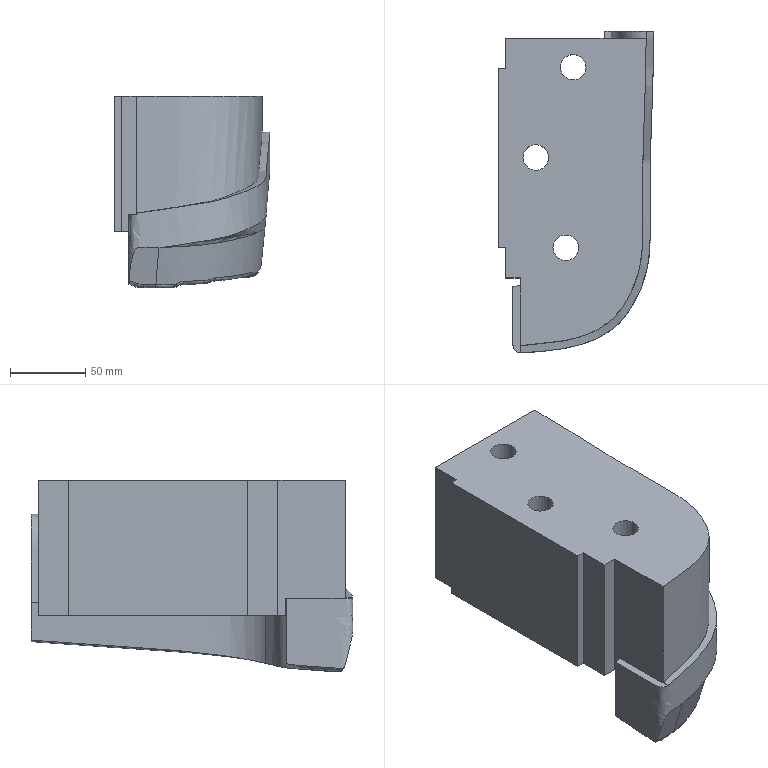Part | NX | features solid 2 | 1 solid | 94 faces | box 103.604 x 213.95 x 127.792 mm | volume 1761546 mm3 | spline 59 | plane 21 | cylinder 14 | commonest cylinder face diameters 17 x3 25 x3 6 x2 10 x2 6.004 x1 10.727 x1